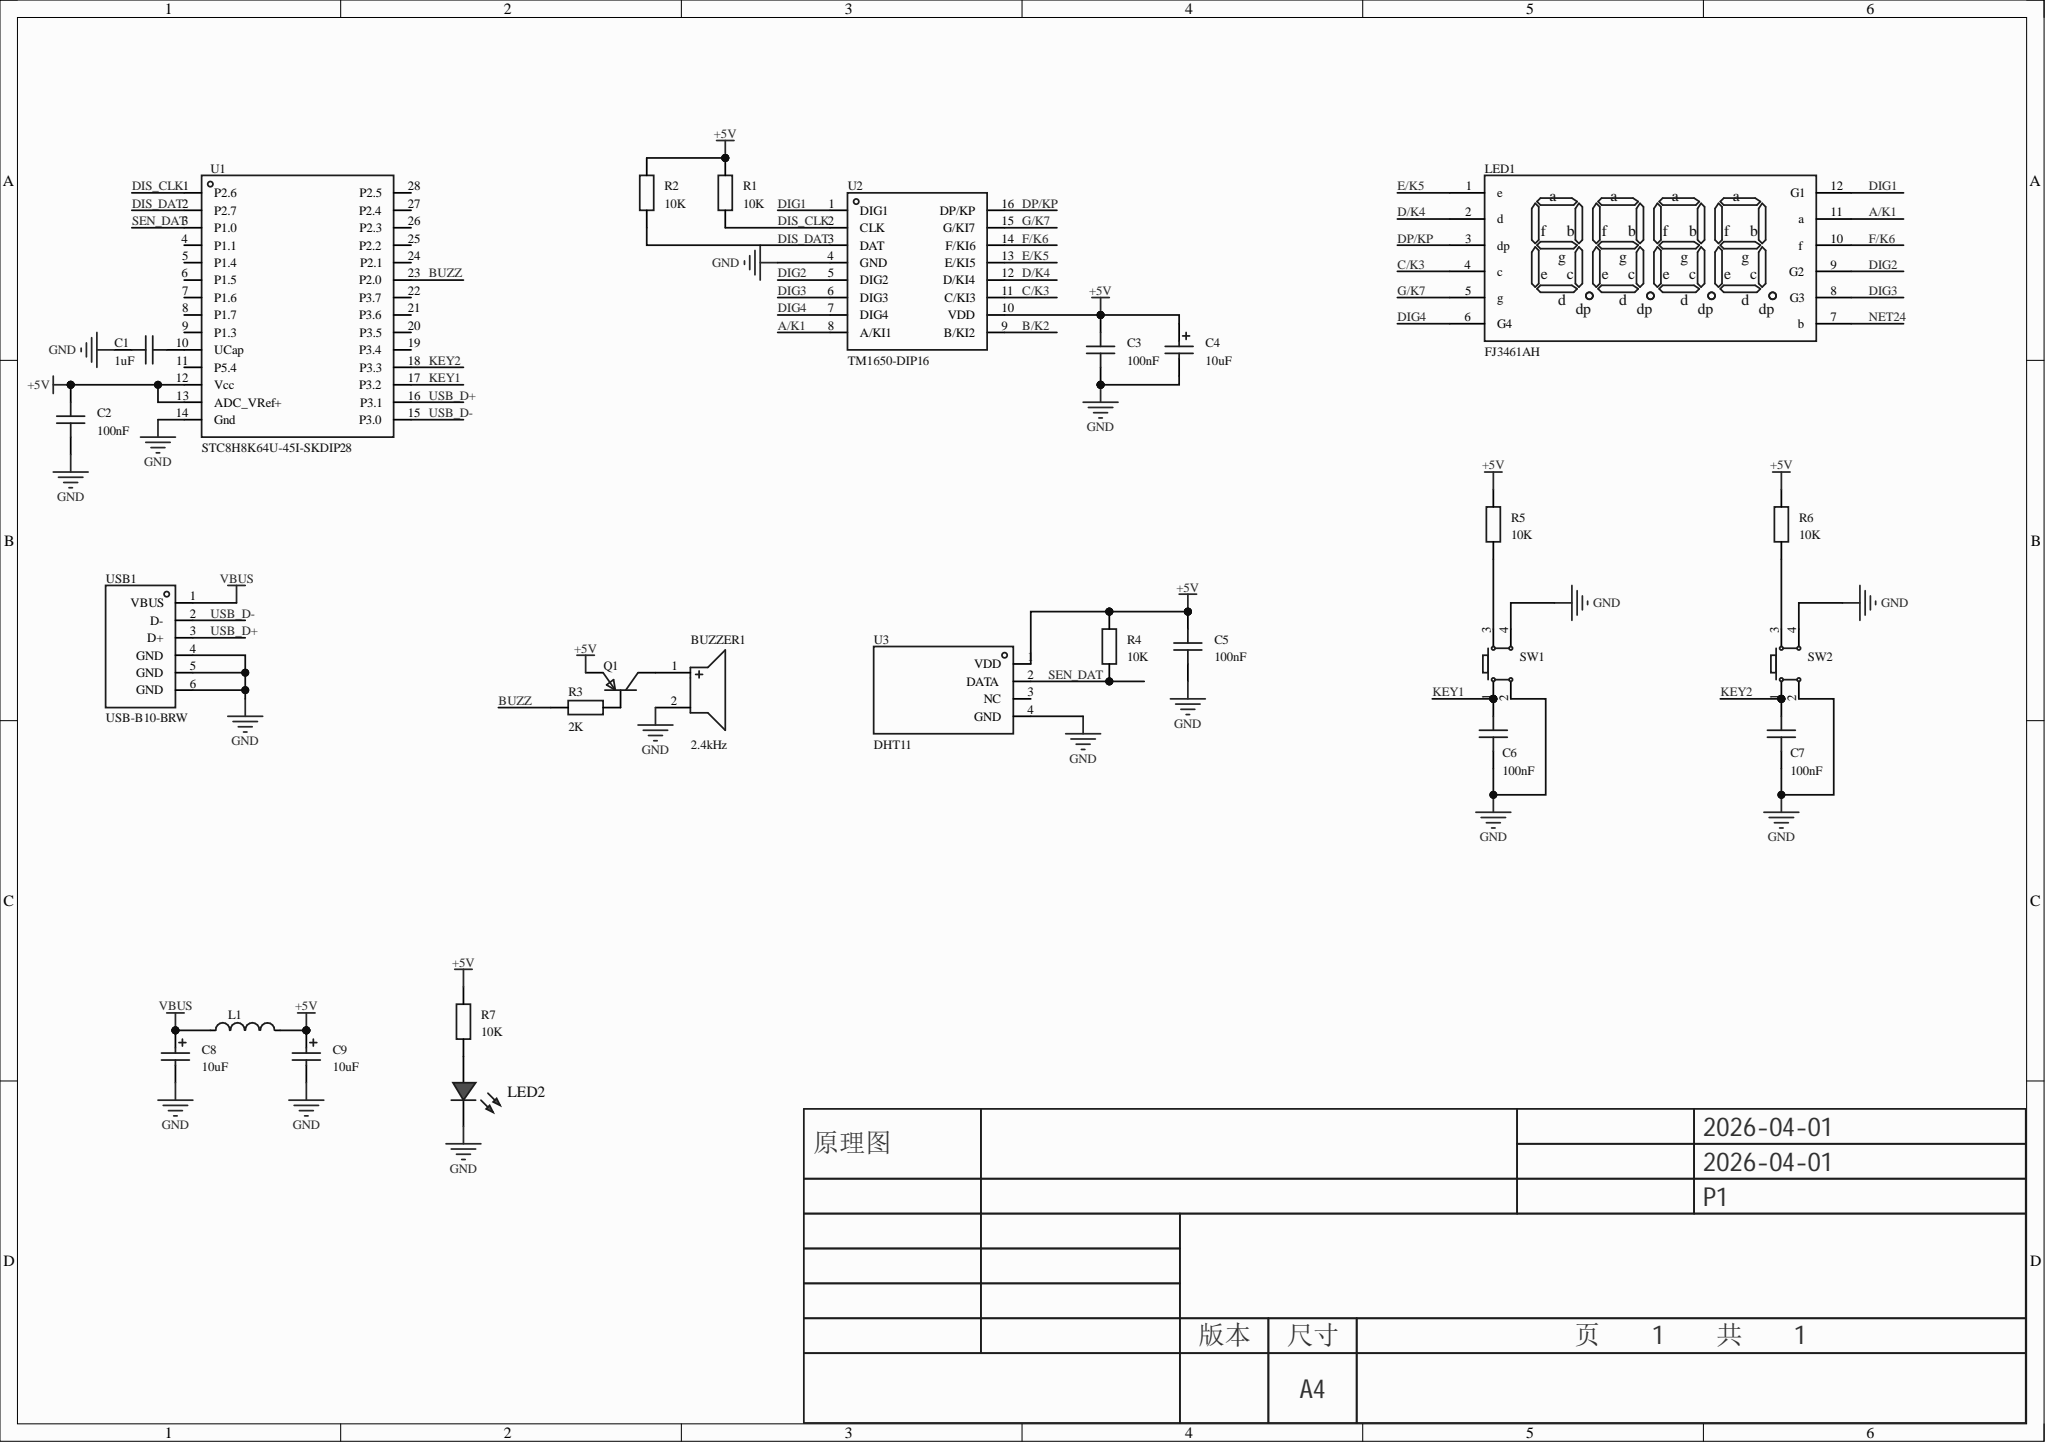Circuit board | Altium Designer | 27 parts | 28 nets
Bill of materials:
Comment,Description,Designator,Footprint,LibRef,Quantity
"2.4kHz","驱动方式:有源(内含驱动线路);构造类型:电磁式;频率:2.4kHz;声压(SPL):88dB;","BUZZER1","BUZ-TH_BD12.0-P7.60-D0.6-FD","TMB12A05","1"
"1uF","","C1","C0603","CAP_0603","1"
"100nF","","C2, C3, C5, C6, C7","C0603","CAP_0603","5"
"10uF","","C4, C8, C9","C_Ele_SMD_3x5.4mm","C_Ele_SMD_3x5.4mm","3"
"10uH","","L1","L0603","L_0603","1"
"FJ3461AH","数码管位数:4位;字符尺寸(英寸):0.36;耗散功率(Pd):-;发光颜色:红色;LED极性:共阴极;","LED1","LED-SEG-TH_12P-L30.0-W14.0-P2.54-S10.16-BL","FJ3461AH","1"
"","","LED2","LED_0603","LED_0603-R","1"
"","","Q1","S8550P_SOT","S8550_SOT_PNP","1"
"10K","","R1, R2, R4, R5, R6, R7","R0603","Res_0603","6"
"2K","","R3","R0603","Res_0603","1"
"","","SW1, SW2","SW-TH_4P-L6.0-W6.0-P4.50-LS6.5","Key_TH_6x6x6","2"
"STC8H8K64U-45I-SKDIP28","","U1","DIP-28_L35.3-W7.3-P2.54-LS8.4-BL","STC8H8K64U-45I-SKDIP28","1"
"TM1650-DIP16","类型:-;工作电压(DC):3V~5.5V;开关频率:-;通道数:-;输出电压:-;输出电流:150mA;调光:-;拓扑结构:-;","U2","DIP-16_L19.3-W6.4-P2.54-LS8.0-BL","TM1650-DIP16","1"
"DHT11","温度范围:-20℃~+60℃;湿度范围:5%RH~95%RH;湿度精度:±5%RH;","U3","SENSOR-TH_DHT11","DHT11","1"
"USB-B10-BRW","连接器类型:Type-B;协议标准:USB 2.0;公母:母;安装方式:弯插;触点数量:4P;端口数量:1;额定电流 - 电源:1.5A;工作温度:-20℃~+70℃;","USB1","USB-B-TH_USB-B10-BRW","USB-B10-BRW","1"
Netlist (Protel format):
[
BUZZER1
BUZ-TH_BD12.0-P7.60-D0.6-FD
2.4kHz



]
[
C1
C0603
1uF



]
[
C2
C0603
100nF



]
[
C3
C0603
100nF



]
[
C4
C_Ele_SMD_3x5.4mm
10uF



]
[
C5
C0603
100nF



]
[
C6
C0603
100nF



]
[
C7
C0603
100nF



]
[
C8
C_Ele_SMD_3x5.4mm
10uF



]
[
C9
C_Ele_SMD_3x5.4mm
10uF



]
[
L1
L0603
10uH



]
[
LED1
LED-SEG-TH_12P-L30.0-W14.0-P2.54-S10.16-BL
FJ3461AH



]
[
LED2
LED_0603




]
[
Q1
S8550P_SOT




]
[
R1
R0603
10K



]
[
R2
R0603
10K



]
[
R3
R0603
2K



]
[
R4
R0603
10K



]
[
R5
R0603
10K



]
[
R6
R0603
10K



]
[
R7
R0603
10K



]
[
SW1
SW-TH_4P-L6.0-W6.0-P4.50-LS6.5




]
[
SW2
SW-TH_4P-L6.0-W6.0-P4.50-LS6.5




]
[
U1
DIP-28_L35.3-W7.3-P2.54-LS8.4-BL
STC8H8K64U-45I-SKDIP28



]
[
U2
DIP-16_L19.3-W6.4-P2.54-LS8.0-BL
TM1650-DIP16



]
[
U3
SENSOR-TH_DHT11
DHT11



]
[
USB1
USB-B-TH_USB-B10-BRW
USB-B10-BRW



]
(
VBUS
C8-1
L1-1
USB1-1
)
(
USB_D-
U1-15
USB1-2
)
(
USB_D+
U1-16
USB1-3
)
(
SEN_DAT
R4-1
U1-3
U3-2
)
(
NetR6_1
R6-1
SW2-3
)
(
NetR5_1
R5-1
SW1-3
)
(
NetQ1_1
Q1-1
R3-2
)
(
NetLED2_2
LED2-2
R7-1
)
(
NetC1_2
C1-2
U1-10
)
(
NetBUZZER1_1
BUZZER1-1
Q1-3
)
(
KEY2
C7-2
SW2-1
U1-18
)
(
KEY1
C6-2
SW1-1
U1-17
)
(
GND
BUZZER1-2
C1-1
C2-1
C3-1
C4-2
C5-1
C6-1
C7-1
C8-2
C9-2
LED2-1
SW1-2
SW1-4
SW2-2
SW2-4
U1-14
U2-4
U3-4
USB1-4
USB1-5
USB1-6
)
(
G/K7
LED1-5
U2-15
)
(
F/K6
LED1-10
U2-14
)
(
E/K5
LED1-1
U2-13
)
(
DP/KP
LED1-3
U2-16
)
(
DIS_DAT
R2-1
U1-2
U2-3
)
(
DIS_CLK
R1-1
U1-1
U2-2
)
(
DIG4
LED1-6
U2-7
)
(
DIG3
LED1-8
U2-6
)
(
DIG2
LED1-9
U2-5
)
(
DIG1
LED1-12
U2-1
)
(
D/K4
LED1-2
U2-12
)
(
C/K3
LED1-4
U2-11
)
(
BUZZ
R3-1
U1-23
)
(
A/K1
LED1-11
U2-8
)
(
+5V
C2-2
C3-2
C4-1
C5-2
C9-1
L1-2
Q1-2
R1-2
R2-2
R4-2
R5-2
R6-2
R7-2
U1-12
U1-13
U2-10
U3-1
)